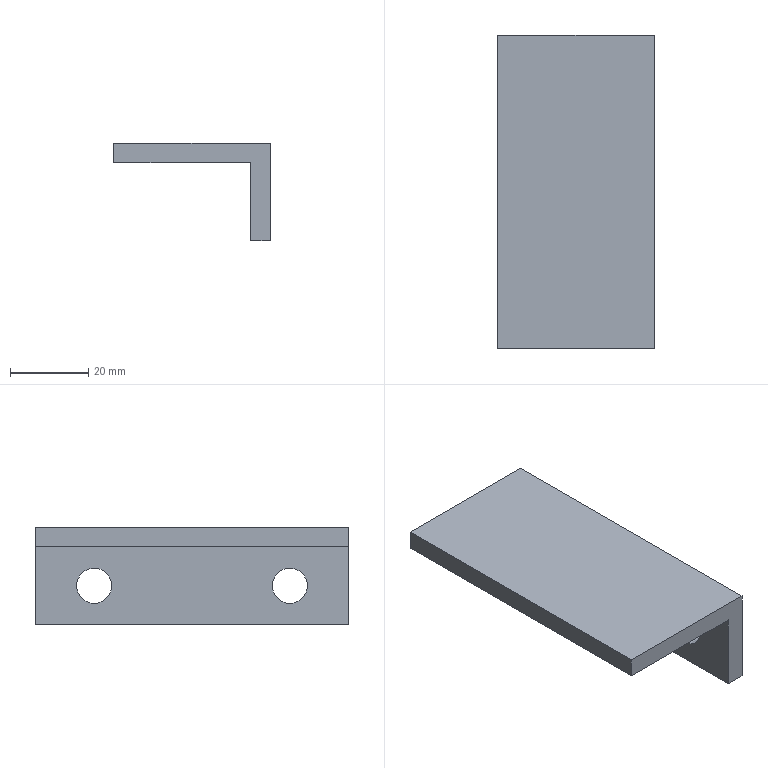Part | STEP file | lll_id4406_x_t | 1 solid | 10 faces | box 40 x 80 x 25 mm | volume 23364 mm3 | plane 8 | cylinder 2 | commonest cylinder face diameters 9 x2
STEP:
#1=CARTESIAN_POINT('',(137.435,-284.1,-8.));
#2=VERTEX_POINT('',#1);
#3=CARTESIAN_POINT('',(137.435,-284.1,-3.));
#4=VERTEX_POINT('',#3);
#5=CARTESIAN_POINT('',(137.435,-284.1,-33.));
#6=DIRECTION('',(0.,0.,1.));
#7=VECTOR('',#6,1.);
#8=LINE('',#5,#7);
#9=EDGE_CURVE('',#2,#4,#8,.T.);
#10=ORIENTED_EDGE('',*,*,#9,.T.);
#11=CARTESIAN_POINT('',(137.435,-204.1,-3.));
#12=VERTEX_POINT('',#11);
#13=CARTESIAN_POINT('',(137.435,48.4,-3.));
#14=DIRECTION('',(0.,1.,0.));
#15=VECTOR('',#14,1.);
#16=LINE('',#13,#15);
#17=EDGE_CURVE('',#4,#12,#16,.T.);
#18=ORIENTED_EDGE('',*,*,#17,.T.);
#19=CARTESIAN_POINT('',(137.435,-204.1,-8.));
#20=VERTEX_POINT('',#19);
#21=CARTESIAN_POINT('',(137.435,-204.1,-33.));
#22=DIRECTION('',(0.,0.,-1.));
#23=VECTOR('',#22,1.);
#24=LINE('',#21,#23);
#25=EDGE_CURVE('',#12,#20,#24,.T.);
#26=ORIENTED_EDGE('',*,*,#25,.T.);
#27=CARTESIAN_POINT('',(137.435,48.4,-8.));
#28=DIRECTION('',(0.,-1.,0.));
#29=VECTOR('',#28,1.);
#30=LINE('',#27,#29);
#31=EDGE_CURVE('',#20,#2,#30,.T.);
#32=ORIENTED_EDGE('',*,*,#31,.T.);
#33=EDGE_LOOP('',(#10,#18,#26,#32));
#34=FACE_OUTER_BOUND('',#33,.T.);
#35=CARTESIAN_POINT('',(137.435,48.4,-33.));
#36=DIRECTION('',(-1.,0.,0.));
#37=DIRECTION('',(0.,0.,-1.));
#38=AXIS2_PLACEMENT_3D('',#35,#36,#37);
#39=PLANE('',#38);
#40=ADVANCED_FACE('',(#34),#39,.T.);
#41=ORIENTED_EDGE('',*,*,#17,.F.);
#42=CARTESIAN_POINT('',(177.435,-284.1,-3.));
#43=VERTEX_POINT('',#42);
#44=CARTESIAN_POINT('',(176.435,-284.1,-3.));
#45=DIRECTION('',(-1.,0.,0.));
#46=VECTOR('',#45,1.);
#47=LINE('',#44,#46);
#48=EDGE_CURVE('',#43,#4,#47,.T.);
#49=ORIENTED_EDGE('',*,*,#48,.F.);
#50=CARTESIAN_POINT('',(177.435,-204.1,-3.));
#51=VERTEX_POINT('',#50);
#52=CARTESIAN_POINT('',(177.435,-244.1,-3.));
#53=DIRECTION('',(0.,-1.,0.));
#54=VECTOR('',#53,1.);
#55=LINE('',#52,#54);
#56=EDGE_CURVE('',#51,#43,#55,.T.);
#57=ORIENTED_EDGE('',*,*,#56,.F.);
#58=CARTESIAN_POINT('',(176.435,-204.1,-3.));
#59=DIRECTION('',(-1.,0.,0.));
#60=VECTOR('',#59,1.);
#61=LINE('',#58,#60);
#62=EDGE_CURVE('',#51,#12,#61,.T.);
#63=ORIENTED_EDGE('',*,*,#62,.T.);
#64=EDGE_LOOP('',(#41,#49,#57,#63));
#65=FACE_OUTER_BOUND('',#64,.T.);
#66=CARTESIAN_POINT('',(176.435,-244.1,-3.));
#67=DIRECTION('',(0.,0.,1.));
#68=DIRECTION('',(-1.,0.,0.));
#69=AXIS2_PLACEMENT_3D('',#66,#67,#68);
#70=PLANE('',#69);
#71=ADVANCED_FACE('',(#65),#70,.T.);
#72=CARTESIAN_POINT('',(177.435,-204.1,-28.));
#73=VERTEX_POINT('',#72);
#74=CARTESIAN_POINT('',(177.435,-204.1,-28.));
#75=DIRECTION('',(0.,0.,-1.));
#76=VECTOR('',#75,1.);
#77=LINE('',#74,#76);
#78=EDGE_CURVE('',#51,#73,#77,.T.);
#79=ORIENTED_EDGE('',*,*,#78,.T.);
#80=CARTESIAN_POINT('',(172.435,-204.1,-28.));
#81=VERTEX_POINT('',#80);
#82=CARTESIAN_POINT('',(174.935,-204.1,-28.));
#83=DIRECTION('',(-1.,0.,0.));
#84=VECTOR('',#83,1.);
#85=LINE('',#82,#84);
#86=EDGE_CURVE('',#73,#81,#85,.T.);
#87=ORIENTED_EDGE('',*,*,#86,.T.);
#88=CARTESIAN_POINT('',(172.435,-204.1,-8.));
#89=VERTEX_POINT('',#88);
#90=CARTESIAN_POINT('',(172.435,-204.1,-28.));
#91=DIRECTION('',(0.,0.,-1.));
#92=VECTOR('',#91,1.);
#93=LINE('',#90,#92);
#94=EDGE_CURVE('',#89,#81,#93,.T.);
#95=ORIENTED_EDGE('',*,*,#94,.F.);
#96=CARTESIAN_POINT('',(176.435,-204.1,-8.));
#97=DIRECTION('',(-1.,0.,0.));
#98=VECTOR('',#97,1.);
#99=LINE('',#96,#98);
#100=EDGE_CURVE('',#89,#20,#99,.T.);
#101=ORIENTED_EDGE('',*,*,#100,.T.);
#102=ORIENTED_EDGE('',*,*,#25,.F.);
#103=ORIENTED_EDGE('',*,*,#62,.F.);
#104=EDGE_LOOP('',(#79,#87,#95,#101,#102,#103));
#105=FACE_OUTER_BOUND('',#104,.T.);
#106=CARTESIAN_POINT('',(176.435,-204.1,-16.64));
#107=DIRECTION('',(0.,1.,0.));
#108=DIRECTION('',(0.,0.,1.));
#109=AXIS2_PLACEMENT_3D('',#106,#107,#108);
#110=PLANE('',#109);
#111=ADVANCED_FACE('',(#105),#110,.T.);
#112=CARTESIAN_POINT('',(177.435,-284.1,-28.));
#113=VERTEX_POINT('',#112);
#114=CARTESIAN_POINT('',(177.435,48.4,-28.));
#115=DIRECTION('',(0.,-1.,0.));
#116=VECTOR('',#115,1.);
#117=LINE('',#114,#116);
#118=EDGE_CURVE('',#73,#113,#117,.T.);
#119=ORIENTED_EDGE('',*,*,#118,.T.);
#120=CARTESIAN_POINT('',(172.435,-284.1,-28.));
#121=VERTEX_POINT('',#120);
#122=CARTESIAN_POINT('',(174.935,-284.1,-28.));
#123=DIRECTION('',(-1.,0.,0.));
#124=VECTOR('',#123,1.);
#125=LINE('',#122,#124);
#126=EDGE_CURVE('',#113,#121,#125,.T.);
#127=ORIENTED_EDGE('',*,*,#126,.T.);
#128=CARTESIAN_POINT('',(172.435,48.4,-28.));
#129=DIRECTION('',(0.,1.,0.));
#130=VECTOR('',#129,1.);
#131=LINE('',#128,#130);
#132=EDGE_CURVE('',#121,#81,#131,.T.);
#133=ORIENTED_EDGE('',*,*,#132,.T.);
#134=ORIENTED_EDGE('',*,*,#86,.F.);
#135=EDGE_LOOP('',(#119,#127,#133,#134));
#136=FACE_OUTER_BOUND('',#135,.T.);
#137=CARTESIAN_POINT('',(174.935,48.4,-28.));
#138=DIRECTION('',(0.,0.,-1.));
#139=DIRECTION('',(1.,0.,0.));
#140=AXIS2_PLACEMENT_3D('',#137,#138,#139);
#141=PLANE('',#140);
#142=ADVANCED_FACE('',(#136),#141,.T.);
#143=CARTESIAN_POINT('',(172.435,-284.1,-8.));
#144=VERTEX_POINT('',#143);
#145=CARTESIAN_POINT('',(172.435,-284.1,-28.));
#146=DIRECTION('',(0.,0.,1.));
#147=VECTOR('',#146,1.);
#148=LINE('',#145,#147);
#149=EDGE_CURVE('',#121,#144,#148,.T.);
#150=ORIENTED_EDGE('',*,*,#149,.F.);
#151=ORIENTED_EDGE('',*,*,#126,.F.);
#152=CARTESIAN_POINT('',(177.435,-284.1,-28.));
#153=DIRECTION('',(0.,0.,1.));
#154=VECTOR('',#153,1.);
#155=LINE('',#152,#154);
#156=EDGE_CURVE('',#113,#43,#155,.T.);
#157=ORIENTED_EDGE('',*,*,#156,.T.);
#158=ORIENTED_EDGE('',*,*,#48,.T.);
#159=ORIENTED_EDGE('',*,*,#9,.F.);
#160=CARTESIAN_POINT('',(176.435,-284.1,-8.));
#161=DIRECTION('',(-1.,0.,0.));
#162=VECTOR('',#161,1.);
#163=LINE('',#160,#162);
#164=EDGE_CURVE('',#144,#2,#163,.T.);
#165=ORIENTED_EDGE('',*,*,#164,.F.);
#166=EDGE_LOOP('',(#150,#151,#157,#158,#159,#165));
#167=FACE_OUTER_BOUND('',#166,.T.);
#168=CARTESIAN_POINT('',(174.935,-284.1,-28.));
#169=DIRECTION('',(0.,-1.,0.));
#170=DIRECTION('',(0.,0.,-1.));
#171=AXIS2_PLACEMENT_3D('',#168,#169,#170);
#172=PLANE('',#171);
#173=ADVANCED_FACE('',(#167),#172,.T.);
#174=ORIENTED_EDGE('',*,*,#164,.T.);
#175=ORIENTED_EDGE('',*,*,#31,.F.);
#176=ORIENTED_EDGE('',*,*,#100,.F.);
#177=CARTESIAN_POINT('',(172.435,-244.1,-8.));
#178=DIRECTION('',(0.,1.,0.));
#179=VECTOR('',#178,1.);
#180=LINE('',#177,#179);
#181=EDGE_CURVE('',#144,#89,#180,.T.);
#182=ORIENTED_EDGE('',*,*,#181,.F.);
#183=EDGE_LOOP('',(#174,#175,#176,#182));
#184=FACE_OUTER_BOUND('',#183,.T.);
#185=CARTESIAN_POINT('',(176.435,-244.1,-8.));
#186=DIRECTION('',(0.,0.,-1.));
#187=DIRECTION('',(1.,0.,0.));
#188=AXIS2_PLACEMENT_3D('',#185,#186,#187);
#189=PLANE('',#188);
#190=ADVANCED_FACE('',(#184),#189,.T.);
#191=CARTESIAN_POINT('',(177.435,-269.1,-13.5));
#192=VERTEX_POINT('',#191);
#193=CARTESIAN_POINT('',(177.435,-269.1,-18.));
#194=DIRECTION('',(-1.,0.,0.));
#195=DIRECTION('',(0.,0.,1.));
#196=AXIS2_PLACEMENT_3D('',#193,#194,#195);
#197=CIRCLE('',#196,4.5);
#198=EDGE_CURVE('',#192,#192,#197,.T.);
#199=ORIENTED_EDGE('',*,*,#198,.F.);
#200=EDGE_LOOP('',(#199));
#201=FACE_BOUND('',#200,.T.);
#202=CARTESIAN_POINT('',(172.435,-269.1,-22.5));
#203=VERTEX_POINT('',#202);
#204=CARTESIAN_POINT('',(172.435,-269.1,-18.));
#205=DIRECTION('',(1.,0.,0.));
#206=DIRECTION('',(0.,0.,-1.));
#207=AXIS2_PLACEMENT_3D('',#204,#205,#206);
#208=CIRCLE('',#207,4.5);
#209=EDGE_CURVE('',#203,#203,#208,.T.);
#210=ORIENTED_EDGE('',*,*,#209,.F.);
#211=EDGE_LOOP('',(#210));
#212=FACE_BOUND('',#211,.T.);
#213=CARTESIAN_POINT('',(185.435,-269.1,-18.));
#214=DIRECTION('',(-1.,0.,0.));
#215=DIRECTION('',(0.,0.,-1.));
#216=AXIS2_PLACEMENT_3D('',#213,#214,#215);
#217=CYLINDRICAL_SURFACE('',#216,4.5);
#218=ADVANCED_FACE('',(#201,#212),#217,.F.);
#219=CARTESIAN_POINT('',(172.435,-219.1,-22.5));
#220=VERTEX_POINT('',#219);
#221=CARTESIAN_POINT('',(172.435,-219.1,-18.));
#222=DIRECTION('',(1.,0.,0.));
#223=DIRECTION('',(0.,0.,-1.));
#224=AXIS2_PLACEMENT_3D('',#221,#222,#223);
#225=CIRCLE('',#224,4.5);
#226=EDGE_CURVE('',#220,#220,#225,.T.);
#227=ORIENTED_EDGE('',*,*,#226,.T.);
#228=EDGE_LOOP('',(#227));
#229=FACE_BOUND('',#228,.T.);
#230=ORIENTED_EDGE('',*,*,#209,.T.);
#231=EDGE_LOOP('',(#230));
#232=FACE_BOUND('',#231,.T.);
#233=ORIENTED_EDGE('',*,*,#181,.T.);
#234=ORIENTED_EDGE('',*,*,#94,.T.);
#235=ORIENTED_EDGE('',*,*,#132,.F.);
#236=ORIENTED_EDGE('',*,*,#149,.T.);
#237=EDGE_LOOP('',(#233,#234,#235,#236));
#238=FACE_BOUND('',#237,.T.);
#239=CARTESIAN_POINT('',(172.435,48.4,-28.));
#240=DIRECTION('',(-1.,0.,0.));
#241=DIRECTION('',(0.,0.,-1.));
#242=AXIS2_PLACEMENT_3D('',#239,#240,#241);
#243=PLANE('',#242);
#244=ADVANCED_FACE('',(#229,#232,#238),#243,.T.);
#245=CARTESIAN_POINT('',(177.435,-219.1,-13.5));
#246=VERTEX_POINT('',#245);
#247=CARTESIAN_POINT('',(177.435,-219.1,-18.));
#248=DIRECTION('',(-1.,0.,0.));
#249=DIRECTION('',(0.,0.,1.));
#250=AXIS2_PLACEMENT_3D('',#247,#248,#249);
#251=CIRCLE('',#250,4.5);
#252=EDGE_CURVE('',#246,#246,#251,.T.);
#253=ORIENTED_EDGE('',*,*,#252,.T.);
#254=EDGE_LOOP('',(#253));
#255=FACE_BOUND('',#254,.T.);
#256=ORIENTED_EDGE('',*,*,#198,.T.);
#257=EDGE_LOOP('',(#256));
#258=FACE_BOUND('',#257,.T.);
#259=ORIENTED_EDGE('',*,*,#156,.F.);
#260=ORIENTED_EDGE('',*,*,#118,.F.);
#261=ORIENTED_EDGE('',*,*,#78,.F.);
#262=ORIENTED_EDGE('',*,*,#56,.T.);
#263=EDGE_LOOP('',(#259,#260,#261,#262));
#264=FACE_BOUND('',#263,.T.);
#265=CARTESIAN_POINT('',(177.435,48.4,-28.));
#266=DIRECTION('',(1.,0.,0.));
#267=DIRECTION('',(0.,0.,1.));
#268=AXIS2_PLACEMENT_3D('',#265,#266,#267);
#269=PLANE('',#268);
#270=ADVANCED_FACE('',(#255,#258,#264),#269,.T.);
#271=ORIENTED_EDGE('',*,*,#252,.F.);
#272=EDGE_LOOP('',(#271));
#273=FACE_BOUND('',#272,.T.);
#274=ORIENTED_EDGE('',*,*,#226,.F.);
#275=EDGE_LOOP('',(#274));
#276=FACE_BOUND('',#275,.T.);
#277=CARTESIAN_POINT('',(185.435,-219.1,-18.));
#278=DIRECTION('',(-1.,0.,0.));
#279=DIRECTION('',(0.,0.,-1.));
#280=AXIS2_PLACEMENT_3D('',#277,#278,#279);
#281=CYLINDRICAL_SURFACE('',#280,4.5);
#282=ADVANCED_FACE('',(#273,#276),#281,.F.);
#283=CLOSED_SHELL('',(#40,#71,#111,#142,#173,#190,#218,#244,#270,#282));
#284=MANIFOLD_SOLID_BREP('',#283);
#285=(LENGTH_UNIT()NAMED_UNIT(*)SI_UNIT(.MILLI.,.METRE.));
#286=UNCERTAINTY_MEASURE_WITH_UNIT(LENGTH_MEASURE(0.00002),#285,'','');
#287=(NAMED_UNIT(*)PLANE_ANGLE_UNIT()SI_UNIT($,.RADIAN.));
#288=PLANE_ANGLE_MEASURE_WITH_UNIT(PLANE_ANGLE_MEASURE(0.01745),#287);
#289=DIMENSIONAL_EXPONENTS(0.,0.,0.,0.,0.,0.,0.);
#290=(CONVERSION_BASED_UNIT('DEGREE',#288)NAMED_UNIT(#289)PLANE_ANGLE_UNIT());
#291=(NAMED_UNIT(*)SI_UNIT($,.STERADIAN.)SOLID_ANGLE_UNIT());
#292=(GEOMETRIC_REPRESENTATION_CONTEXT(3)GLOBAL_UNCERTAINTY_ASSIGNED_CONTEXT((#286))GLOBAL_UNIT_ASSIGNED_CONTEXT((#285,#290,#291))REPRESENTATION_CONTEXT('',''));
#293=ADVANCED_BREP_SHAPE_REPRESENTATION('',(#284),#292);